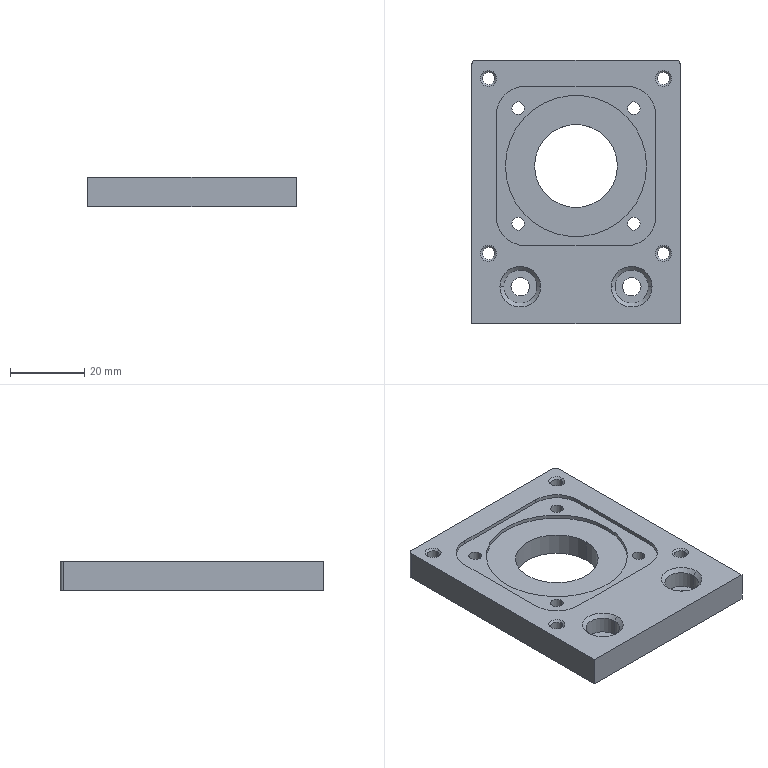Part | SolidWorks | features Chamfer 5, ICE 4, Extrusion 1, HoleWzd 1 | 1 solid | 88 faces | box 56 x 71 x 8 mm | volume 24816 mm3 | cylinder 42 | cone 28 | plane 18 | commonest cylinder face diameters 3.3 x8 3.4 x8 6 x8 5 x4 9 x4 16 x4